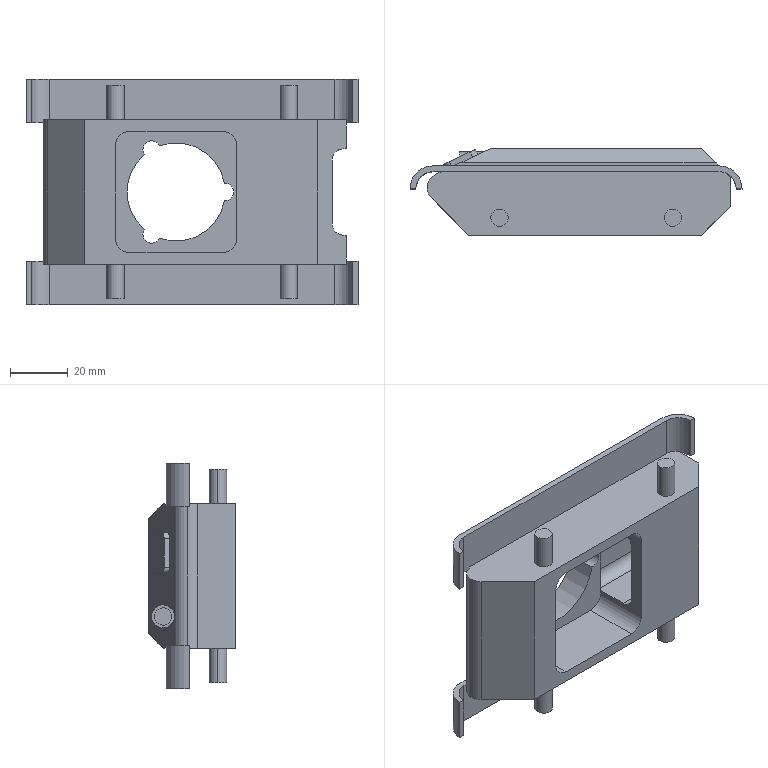Part | SolidWorks | features ICE 9, Chamfer 1, Extrusion 1, MirrorPattern 1 | 1 solid | 118 faces | box 115 x 30 x 78 mm | volume 81134 mm3 | plane 62 | cylinder 56 | commonest cylinder face diameters 4 x16 6 x15 8 x7 10 x6 12 x4 16 x4